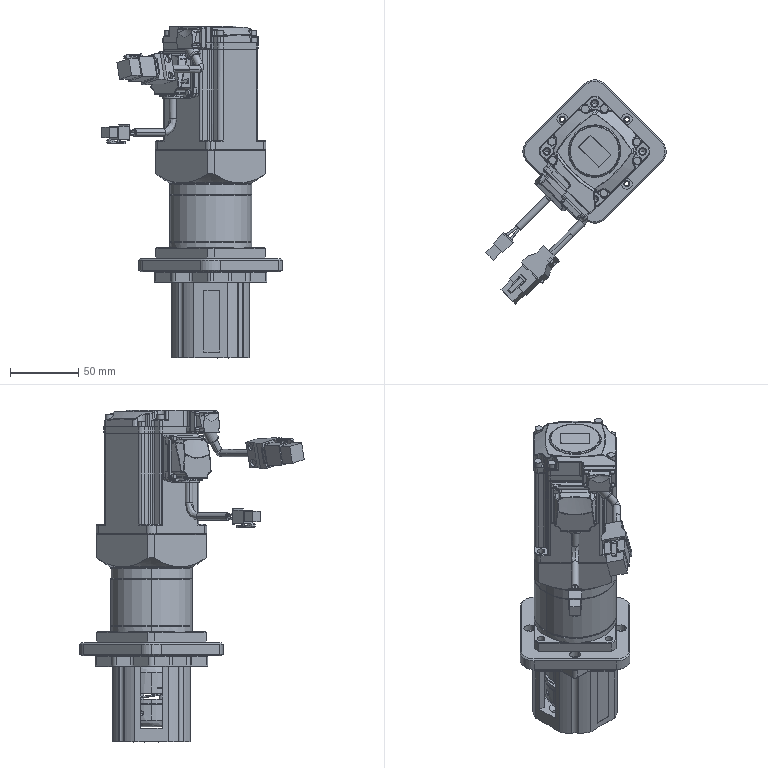Part | STEP file | Copy of 400W gearbox assembly (universal motor base plus Q15)^K50A-1H20-S(formula driven)-L300-motor left- | 13 solids | 1692 faces | box 131.976 x 164.111 x 242.5 mm | volume 719537 mm3 | cylinder 597 | plane 548 | spline 336 | cone 201 | torus 10 | commonest cylinder face diameters 1 x86 4 x48 0.4 x45 6 x44 5.5 x38 3.5 x28